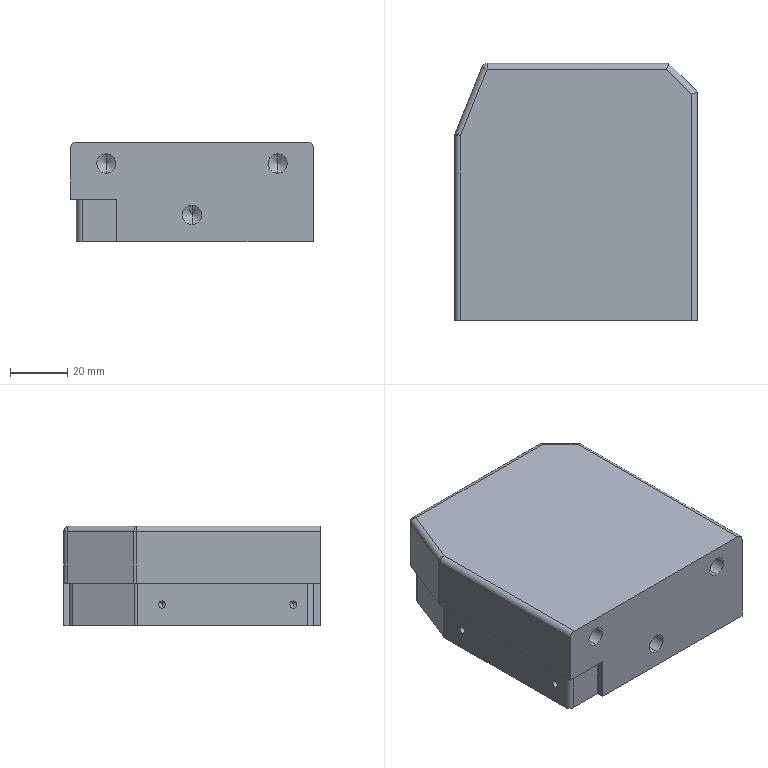Part | STEP file | Guide rail stopper | 1 solid | 67 faces | box 85 x 90 x 35 mm | volume 250787 mm3 | cylinder 27 | plane 22 | cone 16 | sphere 2 | commonest cylinder face diameters 4 x11 2.5 x6 6.8 x6 5.25 x4